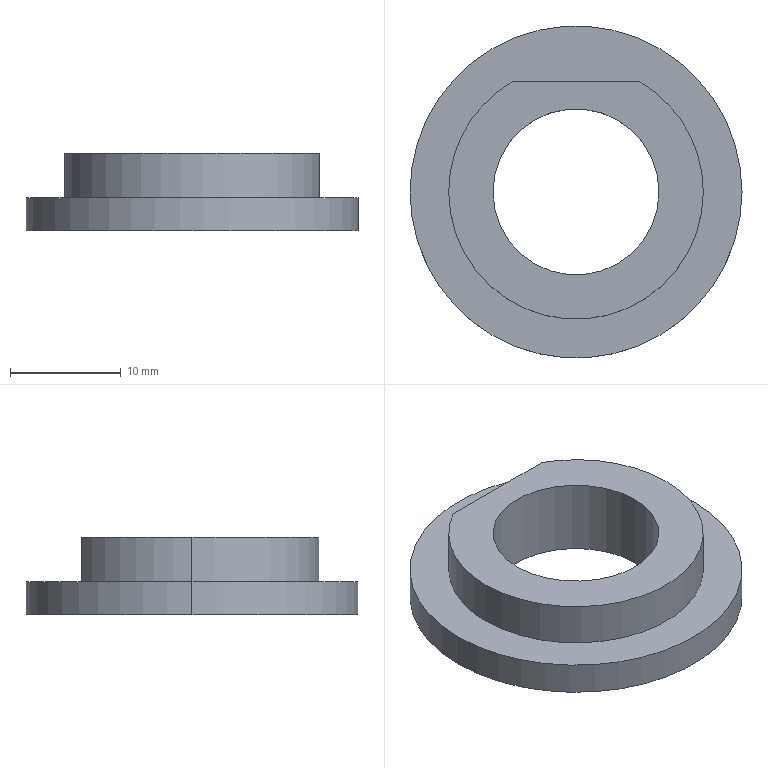Part | SolidWorks | features Extrusion 1, ICE 1 | 1 solid | 11 faces | box 30 x 30 x 7 mm | volume 2499 mm3 | cylinder 7 | plane 4 | commonest cylinder face diameters 23 x3 15 x2 30 x2
STEP:
#1=CARTESIAN_POINT('',(-5.679,10.,3.));
#2=VERTEX_POINT('',#1);
#3=CARTESIAN_POINT('',(-11.5,0.,3.));
#4=VERTEX_POINT('',#3);
#5=CARTESIAN_POINT('',(0.,0.,3.));
#6=DIRECTION('',(0.,0.,1.));
#7=DIRECTION('',(1.,0.,0.));
#8=AXIS2_PLACEMENT_3D('',#5,#6,#7);
#9=CIRCLE('',#8,11.5);
#10=EDGE_CURVE('',#2,#4,#9,.T.);
#11=ORIENTED_EDGE('',*,*,#10,.T.);
#12=CARTESIAN_POINT('',(-11.5,0.,7.));
#13=VERTEX_POINT('',#12);
#14=CARTESIAN_POINT('',(-11.5,0.,3.));
#15=DIRECTION('',(0.,0.,1.));
#16=VECTOR('',#15,1000.);
#17=LINE('',#14,#16);
#18=EDGE_CURVE('',#4,#13,#17,.T.);
#19=ORIENTED_EDGE('',*,*,#18,.T.);
#20=CARTESIAN_POINT('',(-5.679,10.,7.));
#21=VERTEX_POINT('',#20);
#22=CARTESIAN_POINT('',(0.,0.,7.));
#23=DIRECTION('',(0.,0.,1.));
#24=DIRECTION('',(1.,0.,0.));
#25=AXIS2_PLACEMENT_3D('',#22,#23,#24);
#26=CIRCLE('',#25,11.5);
#27=EDGE_CURVE('',#21,#13,#26,.T.);
#28=ORIENTED_EDGE('',*,*,#27,.F.);
#29=CARTESIAN_POINT('',(-5.679,10.,3.));
#30=DIRECTION('',(0.,0.,1.));
#31=VECTOR('',#30,1000.);
#32=LINE('',#29,#31);
#33=EDGE_CURVE('',#2,#21,#32,.T.);
#34=ORIENTED_EDGE('',*,*,#33,.F.);
#35=EDGE_LOOP('',(#11,#19,#28,#34));
#36=FACE_OUTER_BOUND('',#35,.T.);
#37=CARTESIAN_POINT('',(0.,0.,3.));
#38=DIRECTION('',(0.,0.,1.));
#39=DIRECTION('',(1.,0.,0.));
#40=AXIS2_PLACEMENT_3D('',#37,#38,#39);
#41=CYLINDRICAL_SURFACE('',#40,11.5);
#42=ADVANCED_FACE('',(#36),#41,.T.);
#43=ORIENTED_EDGE('',*,*,#18,.F.);
#44=CARTESIAN_POINT('',(11.5,0.,3.));
#45=VERTEX_POINT('',#44);
#46=CARTESIAN_POINT('',(0.,0.,3.));
#47=DIRECTION('',(0.,0.,1.));
#48=DIRECTION('',(1.,0.,0.));
#49=AXIS2_PLACEMENT_3D('',#46,#47,#48);
#50=CIRCLE('',#49,11.5);
#51=EDGE_CURVE('',#4,#45,#50,.T.);
#52=ORIENTED_EDGE('',*,*,#51,.T.);
#53=CARTESIAN_POINT('',(11.5,0.,7.));
#54=VERTEX_POINT('',#53);
#55=CARTESIAN_POINT('',(11.5,0.,3.));
#56=DIRECTION('',(0.,0.,1.));
#57=VECTOR('',#56,1000.);
#58=LINE('',#55,#57);
#59=EDGE_CURVE('',#45,#54,#58,.T.);
#60=ORIENTED_EDGE('',*,*,#59,.T.);
#61=CARTESIAN_POINT('',(0.,0.,7.));
#62=DIRECTION('',(0.,0.,1.));
#63=DIRECTION('',(1.,0.,0.));
#64=AXIS2_PLACEMENT_3D('',#61,#62,#63);
#65=CIRCLE('',#64,11.5);
#66=EDGE_CURVE('',#13,#54,#65,.T.);
#67=ORIENTED_EDGE('',*,*,#66,.F.);
#68=EDGE_LOOP('',(#43,#52,#60,#67));
#69=FACE_OUTER_BOUND('',#68,.T.);
#70=CARTESIAN_POINT('',(0.,0.,3.));
#71=DIRECTION('',(0.,0.,1.));
#72=DIRECTION('',(1.,0.,0.));
#73=AXIS2_PLACEMENT_3D('',#70,#71,#72);
#74=CYLINDRICAL_SURFACE('',#73,11.5);
#75=ADVANCED_FACE('',(#69),#74,.T.);
#76=CARTESIAN_POINT('',(-7.5,0.,7.));
#77=VERTEX_POINT('',#76);
#78=CARTESIAN_POINT('',(7.5,0.,7.));
#79=VERTEX_POINT('',#78);
#80=CARTESIAN_POINT('',(0.,0.,7.));
#81=DIRECTION('',(0.,0.,1.));
#82=DIRECTION('',(1.,0.,0.));
#83=AXIS2_PLACEMENT_3D('',#80,#81,#82);
#84=CIRCLE('',#83,7.5);
#85=EDGE_CURVE('',#77,#79,#84,.T.);
#86=ORIENTED_EDGE('',*,*,#85,.T.);
#87=CARTESIAN_POINT('',(7.5,0.,0.));
#88=VERTEX_POINT('',#87);
#89=CARTESIAN_POINT('',(7.5,0.,7.));
#90=DIRECTION('',(0.,0.,-1.));
#91=VECTOR('',#90,1000.);
#92=LINE('',#89,#91);
#93=EDGE_CURVE('',#79,#88,#92,.T.);
#94=ORIENTED_EDGE('',*,*,#93,.T.);
#95=CARTESIAN_POINT('',(-7.5,0.,0.));
#96=VERTEX_POINT('',#95);
#97=CARTESIAN_POINT('',(0.,0.,0.));
#98=DIRECTION('',(0.,0.,1.));
#99=DIRECTION('',(1.,0.,0.));
#100=AXIS2_PLACEMENT_3D('',#97,#98,#99);
#101=CIRCLE('',#100,7.5);
#102=EDGE_CURVE('',#96,#88,#101,.T.);
#103=ORIENTED_EDGE('',*,*,#102,.F.);
#104=CARTESIAN_POINT('',(-7.5,0.,7.));
#105=DIRECTION('',(0.,0.,-1.));
#106=VECTOR('',#105,1000.);
#107=LINE('',#104,#106);
#108=EDGE_CURVE('',#77,#96,#107,.T.);
#109=ORIENTED_EDGE('',*,*,#108,.F.);
#110=EDGE_LOOP('',(#86,#94,#103,#109));
#111=FACE_OUTER_BOUND('',#110,.T.);
#112=CARTESIAN_POINT('',(0.,0.,7.));
#113=DIRECTION('',(0.,0.,-1.));
#114=DIRECTION('',(-1.,0.,0.));
#115=AXIS2_PLACEMENT_3D('',#112,#113,#114);
#116=CYLINDRICAL_SURFACE('',#115,7.5);
#117=ADVANCED_FACE('',(#111),#116,.F.);
#118=CARTESIAN_POINT('',(15.,0.,3.));
#119=VERTEX_POINT('',#118);
#120=CARTESIAN_POINT('',(-15.,0.,3.));
#121=VERTEX_POINT('',#120);
#122=CARTESIAN_POINT('',(0.,0.,3.));
#123=DIRECTION('',(0.,0.,1.));
#124=DIRECTION('',(1.,0.,0.));
#125=AXIS2_PLACEMENT_3D('',#122,#123,#124);
#126=CIRCLE('',#125,15.);
#127=EDGE_CURVE('',#119,#121,#126,.T.);
#128=ORIENTED_EDGE('',*,*,#127,.F.);
#129=CARTESIAN_POINT('',(15.,0.,0.));
#130=VERTEX_POINT('',#129);
#131=CARTESIAN_POINT('',(15.,0.,7.));
#132=DIRECTION('',(0.,0.,-1.));
#133=VECTOR('',#132,1000.);
#134=LINE('',#131,#133);
#135=EDGE_CURVE('',#119,#130,#134,.T.);
#136=ORIENTED_EDGE('',*,*,#135,.T.);
#137=CARTESIAN_POINT('',(-15.,0.,0.));
#138=VERTEX_POINT('',#137);
#139=CARTESIAN_POINT('',(0.,0.,0.));
#140=DIRECTION('',(0.,0.,1.));
#141=DIRECTION('',(1.,0.,0.));
#142=AXIS2_PLACEMENT_3D('',#139,#140,#141);
#143=CIRCLE('',#142,15.);
#144=EDGE_CURVE('',#130,#138,#143,.T.);
#145=ORIENTED_EDGE('',*,*,#144,.T.);
#146=CARTESIAN_POINT('',(-15.,0.,7.));
#147=DIRECTION('',(0.,0.,-1.));
#148=VECTOR('',#147,1000.);
#149=LINE('',#146,#148);
#150=EDGE_CURVE('',#121,#138,#149,.T.);
#151=ORIENTED_EDGE('',*,*,#150,.F.);
#152=EDGE_LOOP('',(#128,#136,#145,#151));
#153=FACE_OUTER_BOUND('',#152,.T.);
#154=CARTESIAN_POINT('',(0.,0.,7.));
#155=DIRECTION('',(0.,0.,-1.));
#156=DIRECTION('',(-1.,0.,0.));
#157=AXIS2_PLACEMENT_3D('',#154,#155,#156);
#158=CYLINDRICAL_SURFACE('',#157,15.);
#159=ADVANCED_FACE('',(#153),#158,.T.);
#160=ORIENTED_EDGE('',*,*,#85,.F.);
#161=CARTESIAN_POINT('',(0.,0.,7.));
#162=DIRECTION('',(0.,0.,1.));
#163=DIRECTION('',(1.,0.,0.));
#164=AXIS2_PLACEMENT_3D('',#161,#162,#163);
#165=CIRCLE('',#164,7.5);
#166=EDGE_CURVE('',#79,#77,#165,.T.);
#167=ORIENTED_EDGE('',*,*,#166,.F.);
#168=EDGE_LOOP('',(#160,#167));
#169=FACE_BOUND('',#168,.T.);
#170=CARTESIAN_POINT('',(5.679,10.,7.));
#171=VERTEX_POINT('',#170);
#172=CARTESIAN_POINT('',(-5.679,10.,7.));
#173=DIRECTION('',(-1.,0.,0.));
#174=VECTOR('',#173,1000.);
#175=LINE('',#172,#174);
#176=EDGE_CURVE('',#171,#21,#175,.T.);
#177=ORIENTED_EDGE('',*,*,#176,.T.);
#178=ORIENTED_EDGE('',*,*,#27,.T.);
#179=ORIENTED_EDGE('',*,*,#66,.T.);
#180=CARTESIAN_POINT('',(0.,0.,7.));
#181=DIRECTION('',(0.,0.,1.));
#182=DIRECTION('',(1.,0.,0.));
#183=AXIS2_PLACEMENT_3D('',#180,#181,#182);
#184=CIRCLE('',#183,11.5);
#185=EDGE_CURVE('',#54,#171,#184,.T.);
#186=ORIENTED_EDGE('',*,*,#185,.T.);
#187=EDGE_LOOP('',(#177,#178,#179,#186));
#188=FACE_OUTER_BOUND('',#187,.T.);
#189=CARTESIAN_POINT('',(0.,0.,7.));
#190=DIRECTION('',(0.,0.,1.));
#191=DIRECTION('',(1.,0.,0.));
#192=AXIS2_PLACEMENT_3D('',#189,#190,#191);
#193=PLANE('',#192);
#194=ADVANCED_FACE('',(#169,#188),#193,.T.);
#195=ORIENTED_EDGE('',*,*,#135,.F.);
#196=CARTESIAN_POINT('',(0.,0.,3.));
#197=DIRECTION('',(0.,0.,1.));
#198=DIRECTION('',(1.,0.,0.));
#199=AXIS2_PLACEMENT_3D('',#196,#197,#198);
#200=CIRCLE('',#199,15.);
#201=EDGE_CURVE('',#121,#119,#200,.T.);
#202=ORIENTED_EDGE('',*,*,#201,.F.);
#203=ORIENTED_EDGE('',*,*,#150,.T.);
#204=CARTESIAN_POINT('',(0.,0.,0.));
#205=DIRECTION('',(0.,0.,1.));
#206=DIRECTION('',(1.,0.,0.));
#207=AXIS2_PLACEMENT_3D('',#204,#205,#206);
#208=CIRCLE('',#207,15.);
#209=EDGE_CURVE('',#138,#130,#208,.T.);
#210=ORIENTED_EDGE('',*,*,#209,.T.);
#211=EDGE_LOOP('',(#195,#202,#203,#210));
#212=FACE_OUTER_BOUND('',#211,.T.);
#213=CARTESIAN_POINT('',(0.,0.,7.));
#214=DIRECTION('',(0.,0.,-1.));
#215=DIRECTION('',(-1.,0.,0.));
#216=AXIS2_PLACEMENT_3D('',#213,#214,#215);
#217=CYLINDRICAL_SURFACE('',#216,15.);
#218=ADVANCED_FACE('',(#212),#217,.T.);
#219=ORIENTED_EDGE('',*,*,#209,.F.);
#220=ORIENTED_EDGE('',*,*,#144,.F.);
#221=EDGE_LOOP('',(#219,#220));
#222=FACE_OUTER_BOUND('',#221,.T.);
#223=ORIENTED_EDGE('',*,*,#102,.T.);
#224=CARTESIAN_POINT('',(0.,0.,0.));
#225=DIRECTION('',(0.,0.,1.));
#226=DIRECTION('',(1.,0.,0.));
#227=AXIS2_PLACEMENT_3D('',#224,#225,#226);
#228=CIRCLE('',#227,7.5);
#229=EDGE_CURVE('',#88,#96,#228,.T.);
#230=ORIENTED_EDGE('',*,*,#229,.T.);
#231=EDGE_LOOP('',(#223,#230));
#232=FACE_BOUND('',#231,.T.);
#233=CARTESIAN_POINT('',(0.,0.,0.));
#234=DIRECTION('',(0.,0.,1.));
#235=DIRECTION('',(1.,0.,0.));
#236=AXIS2_PLACEMENT_3D('',#233,#234,#235);
#237=PLANE('',#236);
#238=ADVANCED_FACE('',(#222,#232),#237,.F.);
#239=ORIENTED_EDGE('',*,*,#93,.F.);
#240=ORIENTED_EDGE('',*,*,#166,.T.);
#241=ORIENTED_EDGE('',*,*,#108,.T.);
#242=ORIENTED_EDGE('',*,*,#229,.F.);
#243=EDGE_LOOP('',(#239,#240,#241,#242));
#244=FACE_OUTER_BOUND('',#243,.T.);
#245=CARTESIAN_POINT('',(0.,0.,7.));
#246=DIRECTION('',(0.,0.,-1.));
#247=DIRECTION('',(-1.,0.,0.));
#248=AXIS2_PLACEMENT_3D('',#245,#246,#247);
#249=CYLINDRICAL_SURFACE('',#248,7.5);
#250=ADVANCED_FACE('',(#244),#249,.F.);
#251=CARTESIAN_POINT('',(5.679,10.,3.));
#252=VERTEX_POINT('',#251);
#253=CARTESIAN_POINT('',(-5.679,10.,3.));
#254=DIRECTION('',(-1.,0.,0.));
#255=VECTOR('',#254,1000.);
#256=LINE('',#253,#255);
#257=EDGE_CURVE('',#252,#2,#256,.T.);
#258=ORIENTED_EDGE('',*,*,#257,.F.);
#259=CARTESIAN_POINT('',(0.,0.,3.));
#260=DIRECTION('',(0.,0.,1.));
#261=DIRECTION('',(1.,0.,0.));
#262=AXIS2_PLACEMENT_3D('',#259,#260,#261);
#263=CIRCLE('',#262,11.5);
#264=EDGE_CURVE('',#45,#252,#263,.T.);
#265=ORIENTED_EDGE('',*,*,#264,.F.);
#266=ORIENTED_EDGE('',*,*,#51,.F.);
#267=ORIENTED_EDGE('',*,*,#10,.F.);
#268=EDGE_LOOP('',(#258,#265,#266,#267));
#269=FACE_BOUND('',#268,.T.);
#270=ORIENTED_EDGE('',*,*,#201,.T.);
#271=ORIENTED_EDGE('',*,*,#127,.T.);
#272=EDGE_LOOP('',(#270,#271));
#273=FACE_OUTER_BOUND('',#272,.T.);
#274=CARTESIAN_POINT('',(0.,0.,3.));
#275=DIRECTION('',(0.,0.,1.));
#276=DIRECTION('',(1.,0.,0.));
#277=AXIS2_PLACEMENT_3D('',#274,#275,#276);
#278=PLANE('',#277);
#279=ADVANCED_FACE('',(#269,#273),#278,.T.);
#280=ORIENTED_EDGE('',*,*,#59,.F.);
#281=ORIENTED_EDGE('',*,*,#264,.T.);
#282=CARTESIAN_POINT('',(5.679,10.,3.));
#283=DIRECTION('',(0.,0.,1.));
#284=VECTOR('',#283,1000.);
#285=LINE('',#282,#284);
#286=EDGE_CURVE('',#252,#171,#285,.T.);
#287=ORIENTED_EDGE('',*,*,#286,.T.);
#288=ORIENTED_EDGE('',*,*,#185,.F.);
#289=EDGE_LOOP('',(#280,#281,#287,#288));
#290=FACE_OUTER_BOUND('',#289,.T.);
#291=CARTESIAN_POINT('',(0.,0.,3.));
#292=DIRECTION('',(0.,0.,1.));
#293=DIRECTION('',(1.,0.,0.));
#294=AXIS2_PLACEMENT_3D('',#291,#292,#293);
#295=CYLINDRICAL_SURFACE('',#294,11.5);
#296=ADVANCED_FACE('',(#290),#295,.T.);
#297=ORIENTED_EDGE('',*,*,#176,.F.);
#298=ORIENTED_EDGE('',*,*,#286,.F.);
#299=ORIENTED_EDGE('',*,*,#257,.T.);
#300=ORIENTED_EDGE('',*,*,#33,.T.);
#301=EDGE_LOOP('',(#297,#298,#299,#300));
#302=FACE_OUTER_BOUND('',#301,.T.);
#303=CARTESIAN_POINT('',(-5.679,10.,3.));
#304=DIRECTION('',(0.,1.,0.));
#305=DIRECTION('',(-1.,0.,0.));
#306=AXIS2_PLACEMENT_3D('',#303,#304,#305);
#307=PLANE('',#306);
#308=ADVANCED_FACE('',(#302),#307,.T.);
#309=CLOSED_SHELL('',(#42,#75,#117,#159,#194,#218,#238,#250,#279,#296,#308));
#310=MANIFOLD_SOLID_BREP('',#309);
#311=CARTESIAN_POINT('',(0.,0.,0.));
#312=DIRECTION('',(0.,0.,1.));
#313=DIRECTION('',(1.,0.,0.));
#314=AXIS2_PLACEMENT_3D('',#311,#312,#313);
#315=(LENGTH_UNIT()NAMED_UNIT(*)SI_UNIT(.MILLI.,.METRE.));
#316=UNCERTAINTY_MEASURE_WITH_UNIT(LENGTH_MEASURE(0.00001),#315,'','');
#317=(NAMED_UNIT(*)PLANE_ANGLE_UNIT()SI_UNIT($,.RADIAN.));
#318=(NAMED_UNIT(*)SI_UNIT($,.STERADIAN.)SOLID_ANGLE_UNIT());
#319=(GEOMETRIC_REPRESENTATION_CONTEXT(3)GLOBAL_UNCERTAINTY_ASSIGNED_CONTEXT((#316))GLOBAL_UNIT_ASSIGNED_CONTEXT((#315,#317,#318))REPRESENTATION_CONTEXT('',''));
#320=ADVANCED_BREP_SHAPE_REPRESENTATION('',(#310,#314),#319);